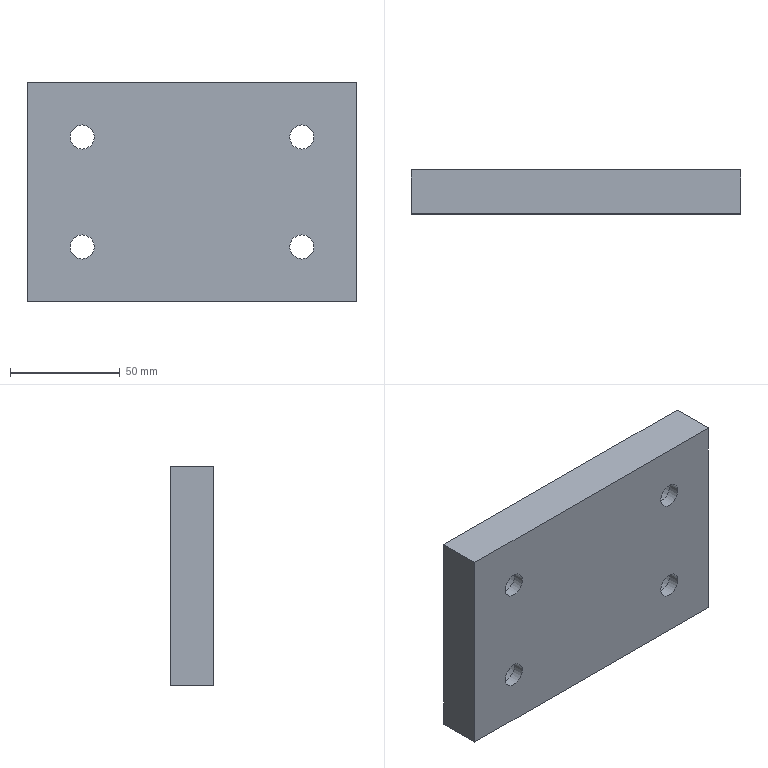Part | NX | features solid 2 | 1 solid | 18 faces | box 150 x 20 x 100 mm | volume 283668 mm3 | plane 10 | cylinder 8 | commonest cylinder face diameters 11 x4 17.5 x4
STEP:
#1=CARTESIAN_POINT('',(950.,815.,-10.));
#2=VERTEX_POINT('',#1);
#3=CARTESIAN_POINT('',(1100.,815.,-10.));
#4=VERTEX_POINT('',#3);
#5=CARTESIAN_POINT('',(1025.,815.,-10.));
#6=DIRECTION('',(1.,0.,0.));
#7=VECTOR('',#6,1000.);
#8=LINE('',#5,#7);
#9=EDGE_CURVE('',#2,#4,#8,.T.);
#10=ORIENTED_EDGE('',*,*,#9,.T.);
#11=CARTESIAN_POINT('',(1100.,835.,-10.));
#12=VERTEX_POINT('',#11);
#13=CARTESIAN_POINT('',(1100.,825.,-10.));
#14=DIRECTION('',(0.,1.,0.));
#15=VECTOR('',#14,1000.);
#16=LINE('',#13,#15);
#17=EDGE_CURVE('',#4,#12,#16,.T.);
#18=ORIENTED_EDGE('',*,*,#17,.T.);
#19=CARTESIAN_POINT('',(950.,835.,-10.));
#20=VERTEX_POINT('',#19);
#21=CARTESIAN_POINT('',(1025.,835.,-10.));
#22=DIRECTION('',(-1.,0.,0.));
#23=VECTOR('',#22,1000.);
#24=LINE('',#21,#23);
#25=EDGE_CURVE('',#12,#20,#24,.T.);
#26=ORIENTED_EDGE('',*,*,#25,.T.);
#27=CARTESIAN_POINT('',(950.,825.,-10.));
#28=DIRECTION('',(0.,-1.,0.));
#29=VECTOR('',#28,1000.);
#30=LINE('',#27,#29);
#31=EDGE_CURVE('',#20,#2,#30,.T.);
#32=ORIENTED_EDGE('',*,*,#31,.T.);
#33=EDGE_LOOP('',(#10,#18,#26,#32));
#34=FACE_BOUND('',#33,.T.);
#35=CARTESIAN_POINT('',(1025.,825.,-10.));
#36=DIRECTION('',(0.,0.,1.));
#37=DIRECTION('',(-1.,0.,0.));
#38=AXIS2_PLACEMENT_3D('',#35,#36,#37);
#39=PLANE('',#38);
#40=ADVANCED_FACE('',(#34),#39,.T.);
#41=CARTESIAN_POINT('',(975.,815.,-29.5));
#42=VERTEX_POINT('',#41);
#43=CARTESIAN_POINT('',(975.,815.,-35.));
#44=DIRECTION('',(0.,-1.,0.));
#45=DIRECTION('',(0.,0.,1.));
#46=AXIS2_PLACEMENT_3D('',#43,#44,#45);
#47=CIRCLE('',#46,5.5);
#48=EDGE_CURVE('',#42,#42,#47,.T.);
#49=ORIENTED_EDGE('',*,*,#48,.F.);
#50=EDGE_LOOP('',(#49));
#51=FACE_BOUND('',#50,.T.);
#52=CARTESIAN_POINT('',(975.,815.,-79.5));
#53=VERTEX_POINT('',#52);
#54=CARTESIAN_POINT('',(975.,815.,-85.));
#55=DIRECTION('',(0.,-1.,0.));
#56=DIRECTION('',(0.,0.,1.));
#57=AXIS2_PLACEMENT_3D('',#54,#55,#56);
#58=CIRCLE('',#57,5.5);
#59=EDGE_CURVE('',#53,#53,#58,.T.);
#60=ORIENTED_EDGE('',*,*,#59,.F.);
#61=EDGE_LOOP('',(#60));
#62=FACE_BOUND('',#61,.T.);
#63=CARTESIAN_POINT('',(1075.,815.,-29.5));
#64=VERTEX_POINT('',#63);
#65=CARTESIAN_POINT('',(1075.,815.,-35.));
#66=DIRECTION('',(0.,-1.,0.));
#67=DIRECTION('',(0.,0.,1.));
#68=AXIS2_PLACEMENT_3D('',#65,#66,#67);
#69=CIRCLE('',#68,5.5);
#70=EDGE_CURVE('',#64,#64,#69,.T.);
#71=ORIENTED_EDGE('',*,*,#70,.F.);
#72=EDGE_LOOP('',(#71));
#73=FACE_BOUND('',#72,.T.);
#74=CARTESIAN_POINT('',(1075.,815.,-79.5));
#75=VERTEX_POINT('',#74);
#76=CARTESIAN_POINT('',(1075.,815.,-85.));
#77=DIRECTION('',(0.,-1.,0.));
#78=DIRECTION('',(0.,0.,1.));
#79=AXIS2_PLACEMENT_3D('',#76,#77,#78);
#80=CIRCLE('',#79,5.5);
#81=EDGE_CURVE('',#75,#75,#80,.T.);
#82=ORIENTED_EDGE('',*,*,#81,.F.);
#83=EDGE_LOOP('',(#82));
#84=FACE_BOUND('',#83,.T.);
#85=CARTESIAN_POINT('',(950.,815.,-110.));
#86=VERTEX_POINT('',#85);
#87=CARTESIAN_POINT('',(950.,815.,-110.));
#88=DIRECTION('',(0.,0.,1.));
#89=VECTOR('',#88,1000.);
#90=LINE('',#87,#89);
#91=EDGE_CURVE('',#86,#2,#90,.T.);
#92=ORIENTED_EDGE('',*,*,#91,.F.);
#93=CARTESIAN_POINT('',(1100.,815.,-110.));
#94=VERTEX_POINT('',#93);
#95=CARTESIAN_POINT('',(1025.,815.,-110.));
#96=DIRECTION('',(-1.,0.,0.));
#97=VECTOR('',#96,1000.);
#98=LINE('',#95,#97);
#99=EDGE_CURVE('',#94,#86,#98,.T.);
#100=ORIENTED_EDGE('',*,*,#99,.F.);
#101=CARTESIAN_POINT('',(1100.,815.,-110.));
#102=DIRECTION('',(0.,0.,1.));
#103=VECTOR('',#102,1000.);
#104=LINE('',#101,#103);
#105=EDGE_CURVE('',#94,#4,#104,.T.);
#106=ORIENTED_EDGE('',*,*,#105,.T.);
#107=ORIENTED_EDGE('',*,*,#9,.F.);
#108=EDGE_LOOP('',(#92,#100,#106,#107));
#109=FACE_BOUND('',#108,.T.);
#110=CARTESIAN_POINT('',(1025.,815.,-110.));
#111=DIRECTION('',(0.,-1.,0.));
#112=DIRECTION('',(0.,0.,-1.));
#113=AXIS2_PLACEMENT_3D('',#110,#111,#112);
#114=PLANE('',#113);
#115=ADVANCED_FACE('',(#51,#62,#73,#84,#109),#114,.T.);
#116=ORIENTED_EDGE('',*,*,#105,.F.);
#117=CARTESIAN_POINT('',(1100.,835.,-110.));
#118=VERTEX_POINT('',#117);
#119=CARTESIAN_POINT('',(1100.,825.,-110.));
#120=DIRECTION('',(0.,-1.,0.));
#121=VECTOR('',#120,1000.);
#122=LINE('',#119,#121);
#123=EDGE_CURVE('',#118,#94,#122,.T.);
#124=ORIENTED_EDGE('',*,*,#123,.F.);
#125=CARTESIAN_POINT('',(1100.,835.,-110.));
#126=DIRECTION('',(0.,0.,1.));
#127=VECTOR('',#126,1000.);
#128=LINE('',#125,#127);
#129=EDGE_CURVE('',#118,#12,#128,.T.);
#130=ORIENTED_EDGE('',*,*,#129,.T.);
#131=ORIENTED_EDGE('',*,*,#17,.F.);
#132=EDGE_LOOP('',(#116,#124,#130,#131));
#133=FACE_BOUND('',#132,.T.);
#134=CARTESIAN_POINT('',(1100.,825.,-110.));
#135=DIRECTION('',(1.,0.,0.));
#136=DIRECTION('',(0.,0.,1.));
#137=AXIS2_PLACEMENT_3D('',#134,#135,#136);
#138=PLANE('',#137);
#139=ADVANCED_FACE('',(#133),#138,.T.);
#140=CARTESIAN_POINT('',(975.,835.,-43.75));
#141=VERTEX_POINT('',#140);
#142=CARTESIAN_POINT('',(975.,835.,-35.));
#143=DIRECTION('',(0.,1.,0.));
#144=DIRECTION('',(0.,0.,-1.));
#145=AXIS2_PLACEMENT_3D('',#142,#143,#144);
#146=CIRCLE('',#145,8.75);
#147=EDGE_CURVE('',#141,#141,#146,.T.);
#148=ORIENTED_EDGE('',*,*,#147,.F.);
#149=EDGE_LOOP('',(#148));
#150=FACE_BOUND('',#149,.T.);
#151=CARTESIAN_POINT('',(975.,835.,-93.75));
#152=VERTEX_POINT('',#151);
#153=CARTESIAN_POINT('',(975.,835.,-85.));
#154=DIRECTION('',(0.,1.,0.));
#155=DIRECTION('',(0.,0.,-1.));
#156=AXIS2_PLACEMENT_3D('',#153,#154,#155);
#157=CIRCLE('',#156,8.75);
#158=EDGE_CURVE('',#152,#152,#157,.T.);
#159=ORIENTED_EDGE('',*,*,#158,.F.);
#160=EDGE_LOOP('',(#159));
#161=FACE_BOUND('',#160,.T.);
#162=CARTESIAN_POINT('',(1075.,835.,-43.75));
#163=VERTEX_POINT('',#162);
#164=CARTESIAN_POINT('',(1075.,835.,-35.));
#165=DIRECTION('',(0.,1.,0.));
#166=DIRECTION('',(0.,0.,-1.));
#167=AXIS2_PLACEMENT_3D('',#164,#165,#166);
#168=CIRCLE('',#167,8.75);
#169=EDGE_CURVE('',#163,#163,#168,.T.);
#170=ORIENTED_EDGE('',*,*,#169,.F.);
#171=EDGE_LOOP('',(#170));
#172=FACE_BOUND('',#171,.T.);
#173=CARTESIAN_POINT('',(1075.,835.,-93.75));
#174=VERTEX_POINT('',#173);
#175=CARTESIAN_POINT('',(1075.,835.,-85.));
#176=DIRECTION('',(0.,1.,0.));
#177=DIRECTION('',(0.,0.,-1.));
#178=AXIS2_PLACEMENT_3D('',#175,#176,#177);
#179=CIRCLE('',#178,8.75);
#180=EDGE_CURVE('',#174,#174,#179,.T.);
#181=ORIENTED_EDGE('',*,*,#180,.F.);
#182=EDGE_LOOP('',(#181));
#183=FACE_BOUND('',#182,.T.);
#184=ORIENTED_EDGE('',*,*,#129,.F.);
#185=CARTESIAN_POINT('',(950.,835.,-110.));
#186=VERTEX_POINT('',#185);
#187=CARTESIAN_POINT('',(1025.,835.,-110.));
#188=DIRECTION('',(1.,0.,0.));
#189=VECTOR('',#188,1000.);
#190=LINE('',#187,#189);
#191=EDGE_CURVE('',#186,#118,#190,.T.);
#192=ORIENTED_EDGE('',*,*,#191,.F.);
#193=CARTESIAN_POINT('',(950.,835.,-110.));
#194=DIRECTION('',(0.,0.,1.));
#195=VECTOR('',#194,1000.);
#196=LINE('',#193,#195);
#197=EDGE_CURVE('',#186,#20,#196,.T.);
#198=ORIENTED_EDGE('',*,*,#197,.T.);
#199=ORIENTED_EDGE('',*,*,#25,.F.);
#200=EDGE_LOOP('',(#184,#192,#198,#199));
#201=FACE_BOUND('',#200,.T.);
#202=CARTESIAN_POINT('',(1025.,835.,-110.));
#203=DIRECTION('',(0.,1.,0.));
#204=DIRECTION('',(0.,0.,1.));
#205=AXIS2_PLACEMENT_3D('',#202,#203,#204);
#206=PLANE('',#205);
#207=ADVANCED_FACE('',(#150,#161,#172,#183,#201),#206,.T.);
#208=CARTESIAN_POINT('',(950.,825.,-110.));
#209=DIRECTION('',(0.,1.,0.));
#210=VECTOR('',#209,1000.);
#211=LINE('',#208,#210);
#212=EDGE_CURVE('',#86,#186,#211,.T.);
#213=ORIENTED_EDGE('',*,*,#212,.T.);
#214=ORIENTED_EDGE('',*,*,#191,.T.);
#215=ORIENTED_EDGE('',*,*,#123,.T.);
#216=ORIENTED_EDGE('',*,*,#99,.T.);
#217=EDGE_LOOP('',(#213,#214,#215,#216));
#218=FACE_BOUND('',#217,.T.);
#219=CARTESIAN_POINT('',(1025.,825.,-110.));
#220=DIRECTION('',(0.,0.,-1.));
#221=DIRECTION('',(1.,0.,0.));
#222=AXIS2_PLACEMENT_3D('',#219,#220,#221);
#223=PLANE('',#222);
#224=ADVANCED_FACE('',(#218),#223,.T.);
#225=ORIENTED_EDGE('',*,*,#212,.F.);
#226=ORIENTED_EDGE('',*,*,#91,.T.);
#227=ORIENTED_EDGE('',*,*,#31,.F.);
#228=ORIENTED_EDGE('',*,*,#197,.F.);
#229=EDGE_LOOP('',(#225,#226,#227,#228));
#230=FACE_BOUND('',#229,.T.);
#231=CARTESIAN_POINT('',(950.,825.,-110.));
#232=DIRECTION('',(-1.,0.,0.));
#233=DIRECTION('',(0.,0.,-1.));
#234=AXIS2_PLACEMENT_3D('',#231,#232,#233);
#235=PLANE('',#234);
#236=ADVANCED_FACE('',(#230),#235,.T.);
#237=CARTESIAN_POINT('',(1075.,820.,-90.5));
#238=VERTEX_POINT('',#237);
#239=CARTESIAN_POINT('',(1075.,820.,-85.));
#240=DIRECTION('',(0.,1.,0.));
#241=DIRECTION('',(0.,0.,-1.));
#242=AXIS2_PLACEMENT_3D('',#239,#240,#241);
#243=CIRCLE('',#242,5.5);
#244=EDGE_CURVE('',#238,#238,#243,.F.);
#245=ORIENTED_EDGE('',*,*,#244,.F.);
#246=EDGE_LOOP('',(#245));
#247=FACE_BOUND('',#246,.T.);
#248=ORIENTED_EDGE('',*,*,#81,.T.);
#249=EDGE_LOOP('',(#248));
#250=FACE_BOUND('',#249,.T.);
#251=CARTESIAN_POINT('',(1075.,815.,-85.));
#252=DIRECTION('',(0.,1.,0.));
#253=DIRECTION('',(0.,0.,1.));
#254=AXIS2_PLACEMENT_3D('',#251,#252,#253);
#255=CYLINDRICAL_SURFACE('',#254,5.5);
#256=ADVANCED_FACE('',(#247,#250),#255,.F.);
#257=CARTESIAN_POINT('',(1075.,820.,-76.25));
#258=VERTEX_POINT('',#257);
#259=CARTESIAN_POINT('',(1075.,820.,-85.));
#260=DIRECTION('',(0.,-1.,0.));
#261=DIRECTION('',(0.,0.,1.));
#262=AXIS2_PLACEMENT_3D('',#259,#260,#261);
#263=CIRCLE('',#262,8.75);
#264=EDGE_CURVE('',#258,#258,#263,.T.);
#265=ORIENTED_EDGE('',*,*,#264,.F.);
#266=EDGE_LOOP('',(#265));
#267=FACE_BOUND('',#266,.T.);
#268=ORIENTED_EDGE('',*,*,#244,.T.);
#269=EDGE_LOOP('',(#268));
#270=FACE_BOUND('',#269,.T.);
#271=CARTESIAN_POINT('',(1075.,820.,-85.));
#272=DIRECTION('',(0.,-1.,0.));
#273=DIRECTION('',(0.,0.,-1.));
#274=AXIS2_PLACEMENT_3D('',#271,#272,#273);
#275=PLANE('',#274);
#276=ADVANCED_FACE('',(#267,#270),#275,.F.);
#277=ORIENTED_EDGE('',*,*,#180,.T.);
#278=EDGE_LOOP('',(#277));
#279=FACE_BOUND('',#278,.T.);
#280=ORIENTED_EDGE('',*,*,#264,.T.);
#281=EDGE_LOOP('',(#280));
#282=FACE_BOUND('',#281,.T.);
#283=CARTESIAN_POINT('',(1075.,820.,-85.));
#284=DIRECTION('',(0.,1.,0.));
#285=DIRECTION('',(0.,0.,1.));
#286=AXIS2_PLACEMENT_3D('',#283,#284,#285);
#287=CYLINDRICAL_SURFACE('',#286,8.75);
#288=ADVANCED_FACE('',(#279,#282),#287,.F.);
#289=CARTESIAN_POINT('',(1075.,820.,-40.5));
#290=VERTEX_POINT('',#289);
#291=CARTESIAN_POINT('',(1075.,820.,-35.));
#292=DIRECTION('',(0.,1.,0.));
#293=DIRECTION('',(0.,0.,-1.));
#294=AXIS2_PLACEMENT_3D('',#291,#292,#293);
#295=CIRCLE('',#294,5.5);
#296=EDGE_CURVE('',#290,#290,#295,.F.);
#297=ORIENTED_EDGE('',*,*,#296,.F.);
#298=EDGE_LOOP('',(#297));
#299=FACE_BOUND('',#298,.T.);
#300=ORIENTED_EDGE('',*,*,#70,.T.);
#301=EDGE_LOOP('',(#300));
#302=FACE_BOUND('',#301,.T.);
#303=CARTESIAN_POINT('',(1075.,815.,-35.));
#304=DIRECTION('',(0.,1.,0.));
#305=DIRECTION('',(0.,0.,1.));
#306=AXIS2_PLACEMENT_3D('',#303,#304,#305);
#307=CYLINDRICAL_SURFACE('',#306,5.5);
#308=ADVANCED_FACE('',(#299,#302),#307,.F.);
#309=CARTESIAN_POINT('',(1075.,820.,-26.25));
#310=VERTEX_POINT('',#309);
#311=CARTESIAN_POINT('',(1075.,820.,-35.));
#312=DIRECTION('',(0.,-1.,0.));
#313=DIRECTION('',(0.,0.,1.));
#314=AXIS2_PLACEMENT_3D('',#311,#312,#313);
#315=CIRCLE('',#314,8.75);
#316=EDGE_CURVE('',#310,#310,#315,.T.);
#317=ORIENTED_EDGE('',*,*,#316,.F.);
#318=EDGE_LOOP('',(#317));
#319=FACE_BOUND('',#318,.T.);
#320=ORIENTED_EDGE('',*,*,#296,.T.);
#321=EDGE_LOOP('',(#320));
#322=FACE_BOUND('',#321,.T.);
#323=CARTESIAN_POINT('',(1075.,820.,-35.));
#324=DIRECTION('',(0.,-1.,0.));
#325=DIRECTION('',(0.,0.,-1.));
#326=AXIS2_PLACEMENT_3D('',#323,#324,#325);
#327=PLANE('',#326);
#328=ADVANCED_FACE('',(#319,#322),#327,.F.);
#329=ORIENTED_EDGE('',*,*,#169,.T.);
#330=EDGE_LOOP('',(#329));
#331=FACE_BOUND('',#330,.T.);
#332=ORIENTED_EDGE('',*,*,#316,.T.);
#333=EDGE_LOOP('',(#332));
#334=FACE_BOUND('',#333,.T.);
#335=CARTESIAN_POINT('',(1075.,820.,-35.));
#336=DIRECTION('',(0.,1.,0.));
#337=DIRECTION('',(0.,0.,1.));
#338=AXIS2_PLACEMENT_3D('',#335,#336,#337);
#339=CYLINDRICAL_SURFACE('',#338,8.75);
#340=ADVANCED_FACE('',(#331,#334),#339,.F.);
#341=CARTESIAN_POINT('',(975.,820.,-90.5));
#342=VERTEX_POINT('',#341);
#343=CARTESIAN_POINT('',(975.,820.,-85.));
#344=DIRECTION('',(0.,1.,0.));
#345=DIRECTION('',(0.,0.,-1.));
#346=AXIS2_PLACEMENT_3D('',#343,#344,#345);
#347=CIRCLE('',#346,5.5);
#348=EDGE_CURVE('',#342,#342,#347,.F.);
#349=ORIENTED_EDGE('',*,*,#348,.F.);
#350=EDGE_LOOP('',(#349));
#351=FACE_BOUND('',#350,.T.);
#352=ORIENTED_EDGE('',*,*,#59,.T.);
#353=EDGE_LOOP('',(#352));
#354=FACE_BOUND('',#353,.T.);
#355=CARTESIAN_POINT('',(975.,815.,-85.));
#356=DIRECTION('',(0.,1.,0.));
#357=DIRECTION('',(0.,0.,1.));
#358=AXIS2_PLACEMENT_3D('',#355,#356,#357);
#359=CYLINDRICAL_SURFACE('',#358,5.5);
#360=ADVANCED_FACE('',(#351,#354),#359,.F.);
#361=CARTESIAN_POINT('',(975.,820.,-76.25));
#362=VERTEX_POINT('',#361);
#363=CARTESIAN_POINT('',(975.,820.,-85.));
#364=DIRECTION('',(0.,-1.,0.));
#365=DIRECTION('',(0.,0.,1.));
#366=AXIS2_PLACEMENT_3D('',#363,#364,#365);
#367=CIRCLE('',#366,8.75);
#368=EDGE_CURVE('',#362,#362,#367,.T.);
#369=ORIENTED_EDGE('',*,*,#368,.F.);
#370=EDGE_LOOP('',(#369));
#371=FACE_BOUND('',#370,.T.);
#372=ORIENTED_EDGE('',*,*,#348,.T.);
#373=EDGE_LOOP('',(#372));
#374=FACE_BOUND('',#373,.T.);
#375=CARTESIAN_POINT('',(975.,820.,-85.));
#376=DIRECTION('',(0.,-1.,0.));
#377=DIRECTION('',(0.,0.,-1.));
#378=AXIS2_PLACEMENT_3D('',#375,#376,#377);
#379=PLANE('',#378);
#380=ADVANCED_FACE('',(#371,#374),#379,.F.);
#381=ORIENTED_EDGE('',*,*,#158,.T.);
#382=EDGE_LOOP('',(#381));
#383=FACE_BOUND('',#382,.T.);
#384=ORIENTED_EDGE('',*,*,#368,.T.);
#385=EDGE_LOOP('',(#384));
#386=FACE_BOUND('',#385,.T.);
#387=CARTESIAN_POINT('',(975.,820.,-85.));
#388=DIRECTION('',(0.,1.,0.));
#389=DIRECTION('',(0.,0.,1.));
#390=AXIS2_PLACEMENT_3D('',#387,#388,#389);
#391=CYLINDRICAL_SURFACE('',#390,8.75);
#392=ADVANCED_FACE('',(#383,#386),#391,.F.);
#393=CARTESIAN_POINT('',(975.,820.,-40.5));
#394=VERTEX_POINT('',#393);
#395=CARTESIAN_POINT('',(975.,820.,-35.));
#396=DIRECTION('',(0.,1.,0.));
#397=DIRECTION('',(0.,0.,-1.));
#398=AXIS2_PLACEMENT_3D('',#395,#396,#397);
#399=CIRCLE('',#398,5.5);
#400=EDGE_CURVE('',#394,#394,#399,.F.);
#401=ORIENTED_EDGE('',*,*,#400,.F.);
#402=EDGE_LOOP('',(#401));
#403=FACE_BOUND('',#402,.T.);
#404=ORIENTED_EDGE('',*,*,#48,.T.);
#405=EDGE_LOOP('',(#404));
#406=FACE_BOUND('',#405,.T.);
#407=CARTESIAN_POINT('',(975.,815.,-35.));
#408=DIRECTION('',(0.,1.,0.));
#409=DIRECTION('',(0.,0.,1.));
#410=AXIS2_PLACEMENT_3D('',#407,#408,#409);
#411=CYLINDRICAL_SURFACE('',#410,5.5);
#412=ADVANCED_FACE('',(#403,#406),#411,.F.);
#413=CARTESIAN_POINT('',(975.,820.,-26.25));
#414=VERTEX_POINT('',#413);
#415=CARTESIAN_POINT('',(975.,820.,-35.));
#416=DIRECTION('',(0.,-1.,0.));
#417=DIRECTION('',(0.,0.,1.));
#418=AXIS2_PLACEMENT_3D('',#415,#416,#417);
#419=CIRCLE('',#418,8.75);
#420=EDGE_CURVE('',#414,#414,#419,.T.);
#421=ORIENTED_EDGE('',*,*,#420,.F.);
#422=EDGE_LOOP('',(#421));
#423=FACE_BOUND('',#422,.T.);
#424=ORIENTED_EDGE('',*,*,#400,.T.);
#425=EDGE_LOOP('',(#424));
#426=FACE_BOUND('',#425,.T.);
#427=CARTESIAN_POINT('',(975.,820.,-35.));
#428=DIRECTION('',(0.,-1.,0.));
#429=DIRECTION('',(0.,0.,-1.));
#430=AXIS2_PLACEMENT_3D('',#427,#428,#429);
#431=PLANE('',#430);
#432=ADVANCED_FACE('',(#423,#426),#431,.F.);
#433=ORIENTED_EDGE('',*,*,#147,.T.);
#434=EDGE_LOOP('',(#433));
#435=FACE_BOUND('',#434,.T.);
#436=ORIENTED_EDGE('',*,*,#420,.T.);
#437=EDGE_LOOP('',(#436));
#438=FACE_BOUND('',#437,.T.);
#439=CARTESIAN_POINT('',(975.,820.,-35.));
#440=DIRECTION('',(0.,1.,0.));
#441=DIRECTION('',(0.,0.,1.));
#442=AXIS2_PLACEMENT_3D('',#439,#440,#441);
#443=CYLINDRICAL_SURFACE('',#442,8.75);
#444=ADVANCED_FACE('',(#435,#438),#443,.F.);
#445=CLOSED_SHELL('',(#40,#115,#139,#207,#224,#236,#256,#276,#288,#308,#328,#340,#360,#380,#392,#412,#432,#444));
#446=MANIFOLD_SOLID_BREP('',#445);
#447=(LENGTH_UNIT()NAMED_UNIT(*)SI_UNIT(.MILLI.,.METRE.));
#448=UNCERTAINTY_MEASURE_WITH_UNIT(LENGTH_MEASURE(0.00001),#447,'','');
#449=(NAMED_UNIT(*)PLANE_ANGLE_UNIT()SI_UNIT($,.RADIAN.));
#450=(NAMED_UNIT(*)SI_UNIT($,.STERADIAN.)SOLID_ANGLE_UNIT());
#451=(GEOMETRIC_REPRESENTATION_CONTEXT(3)GLOBAL_UNCERTAINTY_ASSIGNED_CONTEXT((#448))GLOBAL_UNIT_ASSIGNED_CONTEXT((#447,#449,#450))REPRESENTATION_CONTEXT('',''));
#452=ADVANCED_BREP_SHAPE_REPRESENTATION('',(#446),#451);